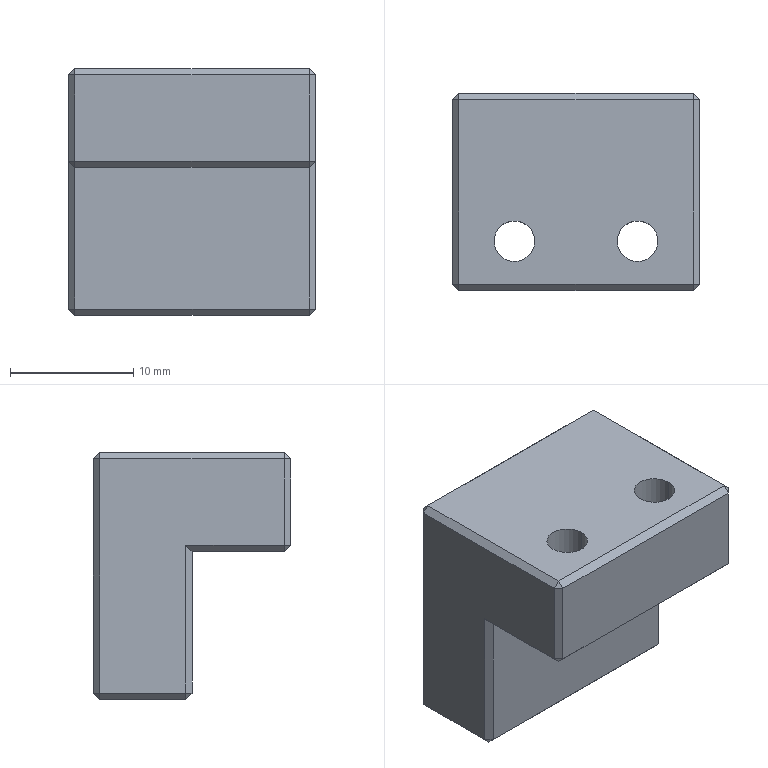Part | SolidWorks | features HoleWzd 2, Chamfer 1, Extrusion 1, ICE 1 | 1 solid | 47 faces | box 20 x 16 x 20 mm | volume 4067 mm3 | plane 35 | cylinder 8 | cone 4 | commonest cylinder face diameters 3.3 x8
STEP:
#1=CARTESIAN_POINT('',(-6.65,-4.,2.));
#2=VERTEX_POINT('',#1);
#3=CARTESIAN_POINT('',(-3.35,-4.,2.));
#4=VERTEX_POINT('',#3);
#5=CARTESIAN_POINT('',(-5.,-4.,2.));
#6=DIRECTION('',(0.,0.,1.));
#7=DIRECTION('',(1.,0.,0.));
#8=AXIS2_PLACEMENT_3D('',#5,#6,#7);
#9=CIRCLE('',#8,1.65);
#10=EDGE_CURVE('',#2,#4,#9,.T.);
#11=ORIENTED_EDGE('',*,*,#10,.F.);
#12=CARTESIAN_POINT('',(-6.65,-4.,10.));
#13=VERTEX_POINT('',#12);
#14=CARTESIAN_POINT('',(-6.65,-4.,10.));
#15=DIRECTION('',(0.,0.,1.));
#16=VECTOR('',#15,1000.);
#17=LINE('',#14,#16);
#18=EDGE_CURVE('',#2,#13,#17,.T.);
#19=ORIENTED_EDGE('',*,*,#18,.T.);
#20=CARTESIAN_POINT('',(-3.35,-4.,10.));
#21=VERTEX_POINT('',#20);
#22=CARTESIAN_POINT('',(-5.,-4.,10.));
#23=DIRECTION('',(0.,0.,1.));
#24=DIRECTION('',(1.,0.,0.));
#25=AXIS2_PLACEMENT_3D('',#22,#23,#24);
#26=CIRCLE('',#25,1.65);
#27=EDGE_CURVE('',#13,#21,#26,.T.);
#28=ORIENTED_EDGE('',*,*,#27,.T.);
#29=CARTESIAN_POINT('',(-3.35,-4.,10.));
#30=DIRECTION('',(0.,0.,1.));
#31=VECTOR('',#30,1000.);
#32=LINE('',#29,#31);
#33=EDGE_CURVE('',#4,#21,#32,.T.);
#34=ORIENTED_EDGE('',*,*,#33,.F.);
#35=EDGE_LOOP('',(#11,#19,#28,#34));
#36=FACE_OUTER_BOUND('',#35,.T.);
#37=CARTESIAN_POINT('',(-5.,-4.,10.));
#38=DIRECTION('',(0.,0.,1.));
#39=DIRECTION('',(1.,0.,0.));
#40=AXIS2_PLACEMENT_3D('',#37,#38,#39);
#41=CYLINDRICAL_SURFACE('',#40,1.65);
#42=ADVANCED_FACE('',(#36),#41,.F.);
#43=CARTESIAN_POINT('',(3.35,-4.,2.));
#44=VERTEX_POINT('',#43);
#45=CARTESIAN_POINT('',(6.65,-4.,2.));
#46=VERTEX_POINT('',#45);
#47=CARTESIAN_POINT('',(5.,-4.,2.));
#48=DIRECTION('',(0.,0.,1.));
#49=DIRECTION('',(1.,0.,0.));
#50=AXIS2_PLACEMENT_3D('',#47,#48,#49);
#51=CIRCLE('',#50,1.65);
#52=EDGE_CURVE('',#44,#46,#51,.T.);
#53=ORIENTED_EDGE('',*,*,#52,.F.);
#54=CARTESIAN_POINT('',(3.35,-4.,10.));
#55=VERTEX_POINT('',#54);
#56=CARTESIAN_POINT('',(3.35,-4.,10.));
#57=DIRECTION('',(0.,0.,1.));
#58=VECTOR('',#57,1000.);
#59=LINE('',#56,#58);
#60=EDGE_CURVE('',#44,#55,#59,.T.);
#61=ORIENTED_EDGE('',*,*,#60,.T.);
#62=CARTESIAN_POINT('',(6.65,-4.,10.));
#63=VERTEX_POINT('',#62);
#64=CARTESIAN_POINT('',(5.,-4.,10.));
#65=DIRECTION('',(0.,0.,1.));
#66=DIRECTION('',(1.,0.,0.));
#67=AXIS2_PLACEMENT_3D('',#64,#65,#66);
#68=CIRCLE('',#67,1.65);
#69=EDGE_CURVE('',#55,#63,#68,.T.);
#70=ORIENTED_EDGE('',*,*,#69,.T.);
#71=CARTESIAN_POINT('',(6.65,-4.,10.));
#72=DIRECTION('',(0.,0.,1.));
#73=VECTOR('',#72,1000.);
#74=LINE('',#71,#73);
#75=EDGE_CURVE('',#46,#63,#74,.T.);
#76=ORIENTED_EDGE('',*,*,#75,.F.);
#77=EDGE_LOOP('',(#53,#61,#70,#76));
#78=FACE_OUTER_BOUND('',#77,.T.);
#79=CARTESIAN_POINT('',(5.,-4.,10.));
#80=DIRECTION('',(0.,0.,1.));
#81=DIRECTION('',(1.,0.,0.));
#82=AXIS2_PLACEMENT_3D('',#79,#80,#81);
#83=CYLINDRICAL_SURFACE('',#82,1.65);
#84=ADVANCED_FACE('',(#78),#83,.F.);
#85=CARTESIAN_POINT('',(-4.1,4.,-3.35));
#86=VERTEX_POINT('',#85);
#87=CARTESIAN_POINT('',(-4.1,4.,-6.65));
#88=VERTEX_POINT('',#87);
#89=CARTESIAN_POINT('',(-4.1,4.,-5.));
#90=DIRECTION('',(1.,0.,0.));
#91=DIRECTION('',(0.,0.,-1.));
#92=AXIS2_PLACEMENT_3D('',#89,#90,#91);
#93=CIRCLE('',#92,1.65);
#94=EDGE_CURVE('',#86,#88,#93,.T.);
#95=ORIENTED_EDGE('',*,*,#94,.F.);
#96=CARTESIAN_POINT('',(10.,4.,-3.35));
#97=VERTEX_POINT('',#96);
#98=CARTESIAN_POINT('',(10.,4.,-3.35));
#99=DIRECTION('',(1.,0.,0.));
#100=VECTOR('',#99,1000.);
#101=LINE('',#98,#100);
#102=EDGE_CURVE('',#86,#97,#101,.T.);
#103=ORIENTED_EDGE('',*,*,#102,.T.);
#104=CARTESIAN_POINT('',(10.,4.,-6.65));
#105=VERTEX_POINT('',#104);
#106=CARTESIAN_POINT('',(10.,4.,-5.));
#107=DIRECTION('',(1.,0.,0.));
#108=DIRECTION('',(0.,0.,-1.));
#109=AXIS2_PLACEMENT_3D('',#106,#107,#108);
#110=CIRCLE('',#109,1.65);
#111=EDGE_CURVE('',#97,#105,#110,.T.);
#112=ORIENTED_EDGE('',*,*,#111,.T.);
#113=CARTESIAN_POINT('',(10.,4.,-6.65));
#114=DIRECTION('',(1.,0.,0.));
#115=VECTOR('',#114,1000.);
#116=LINE('',#113,#115);
#117=EDGE_CURVE('',#88,#105,#116,.T.);
#118=ORIENTED_EDGE('',*,*,#117,.F.);
#119=EDGE_LOOP('',(#95,#103,#112,#118));
#120=FACE_OUTER_BOUND('',#119,.T.);
#121=CARTESIAN_POINT('',(10.,4.,-5.));
#122=DIRECTION('',(1.,0.,0.));
#123=DIRECTION('',(0.,0.,-1.));
#124=AXIS2_PLACEMENT_3D('',#121,#122,#123);
#125=CYLINDRICAL_SURFACE('',#124,1.65);
#126=ADVANCED_FACE('',(#120),#125,.F.);
#127=CARTESIAN_POINT('',(-5.091,4.,-5.));
#128=VERTEX_POINT('',#127);
#129=CARTESIAN_POINT('',(-4.1,4.,-6.65));
#130=DIRECTION('',(0.515,0.,-0.8572));
#131=VECTOR('',#130,1000.);
#132=LINE('',#129,#131);
#133=EDGE_CURVE('',#128,#88,#132,.T.);
#134=ORIENTED_EDGE('',*,*,#133,.F.);
#135=CARTESIAN_POINT('',(-4.1,4.,-3.35));
#136=DIRECTION('',(0.515,0.,0.8572));
#137=VECTOR('',#136,1000.);
#138=LINE('',#135,#137);
#139=EDGE_CURVE('',#128,#86,#138,.T.);
#140=ORIENTED_EDGE('',*,*,#139,.T.);
#141=ORIENTED_EDGE('',*,*,#94,.T.);
#142=EDGE_LOOP('',(#134,#140,#141));
#143=FACE_OUTER_BOUND('',#142,.T.);
#144=CARTESIAN_POINT('',(-4.1,4.,-5.));
#145=DIRECTION('',(1.,0.,0.));
#146=DIRECTION('',(0.,0.,-1.));
#147=AXIS2_PLACEMENT_3D('',#144,#145,#146);
#148=CONICAL_SURFACE('',#147,1.65,1.03);
#149=ADVANCED_FACE('',(#143),#148,.F.);
#150=CARTESIAN_POINT('',(-4.1,4.,6.65));
#151=VERTEX_POINT('',#150);
#152=CARTESIAN_POINT('',(-4.1,4.,3.35));
#153=VERTEX_POINT('',#152);
#154=CARTESIAN_POINT('',(-4.1,4.,5.));
#155=DIRECTION('',(1.,0.,0.));
#156=DIRECTION('',(0.,0.,-1.));
#157=AXIS2_PLACEMENT_3D('',#154,#155,#156);
#158=CIRCLE('',#157,1.65);
#159=EDGE_CURVE('',#151,#153,#158,.T.);
#160=ORIENTED_EDGE('',*,*,#159,.F.);
#161=CARTESIAN_POINT('',(10.,4.,6.65));
#162=VERTEX_POINT('',#161);
#163=CARTESIAN_POINT('',(10.,4.,6.65));
#164=DIRECTION('',(1.,0.,0.));
#165=VECTOR('',#164,1000.);
#166=LINE('',#163,#165);
#167=EDGE_CURVE('',#151,#162,#166,.T.);
#168=ORIENTED_EDGE('',*,*,#167,.T.);
#169=CARTESIAN_POINT('',(10.,4.,3.35));
#170=VERTEX_POINT('',#169);
#171=CARTESIAN_POINT('',(10.,4.,5.));
#172=DIRECTION('',(1.,0.,0.));
#173=DIRECTION('',(0.,0.,-1.));
#174=AXIS2_PLACEMENT_3D('',#171,#172,#173);
#175=CIRCLE('',#174,1.65);
#176=EDGE_CURVE('',#162,#170,#175,.T.);
#177=ORIENTED_EDGE('',*,*,#176,.T.);
#178=CARTESIAN_POINT('',(10.,4.,3.35));
#179=DIRECTION('',(1.,0.,0.));
#180=VECTOR('',#179,1000.);
#181=LINE('',#178,#180);
#182=EDGE_CURVE('',#153,#170,#181,.T.);
#183=ORIENTED_EDGE('',*,*,#182,.F.);
#184=EDGE_LOOP('',(#160,#168,#177,#183));
#185=FACE_OUTER_BOUND('',#184,.T.);
#186=CARTESIAN_POINT('',(10.,4.,5.));
#187=DIRECTION('',(1.,0.,0.));
#188=DIRECTION('',(0.,0.,-1.));
#189=AXIS2_PLACEMENT_3D('',#186,#187,#188);
#190=CYLINDRICAL_SURFACE('',#189,1.65);
#191=ADVANCED_FACE('',(#185),#190,.F.);
#192=CARTESIAN_POINT('',(-5.091,4.,5.));
#193=VERTEX_POINT('',#192);
#194=CARTESIAN_POINT('',(-4.1,4.,3.35));
#195=DIRECTION('',(0.515,0.,-0.8572));
#196=VECTOR('',#195,1000.);
#197=LINE('',#194,#196);
#198=EDGE_CURVE('',#193,#153,#197,.T.);
#199=ORIENTED_EDGE('',*,*,#198,.F.);
#200=CARTESIAN_POINT('',(-4.1,4.,6.65));
#201=DIRECTION('',(0.515,0.,0.8572));
#202=VECTOR('',#201,1000.);
#203=LINE('',#200,#202);
#204=EDGE_CURVE('',#193,#151,#203,.T.);
#205=ORIENTED_EDGE('',*,*,#204,.T.);
#206=ORIENTED_EDGE('',*,*,#159,.T.);
#207=EDGE_LOOP('',(#199,#205,#206));
#208=FACE_OUTER_BOUND('',#207,.T.);
#209=CARTESIAN_POINT('',(-4.1,4.,5.));
#210=DIRECTION('',(1.,0.,0.));
#211=DIRECTION('',(0.,0.,-1.));
#212=AXIS2_PLACEMENT_3D('',#209,#210,#211);
#213=CONICAL_SURFACE('',#212,1.65,1.03);
#214=ADVANCED_FACE('',(#208),#213,.F.);
#215=CARTESIAN_POINT('',(10.,-7.5,2.5));
#216=VERTEX_POINT('',#215);
#217=CARTESIAN_POINT('',(10.,0.5,2.5));
#218=VERTEX_POINT('',#217);
#219=CARTESIAN_POINT('',(10.,8.,2.5));
#220=DIRECTION('',(0.,1.,0.));
#221=VECTOR('',#220,1000.);
#222=LINE('',#219,#221);
#223=EDGE_CURVE('',#216,#218,#222,.T.);
#224=ORIENTED_EDGE('',*,*,#223,.T.);
#225=CARTESIAN_POINT('',(10.,0.5,-9.5));
#226=VERTEX_POINT('',#225);
#227=CARTESIAN_POINT('',(10.,0.5,-10.));
#228=DIRECTION('',(0.,0.,-1.));
#229=VECTOR('',#228,1000.);
#230=LINE('',#227,#229);
#231=EDGE_CURVE('',#218,#226,#230,.T.);
#232=ORIENTED_EDGE('',*,*,#231,.T.);
#233=CARTESIAN_POINT('',(10.,7.5,-9.5));
#234=VERTEX_POINT('',#233);
#235=CARTESIAN_POINT('',(10.,8.,-9.5));
#236=DIRECTION('',(0.,1.,0.));
#237=VECTOR('',#236,1000.);
#238=LINE('',#235,#237);
#239=EDGE_CURVE('',#226,#234,#238,.T.);
#240=ORIENTED_EDGE('',*,*,#239,.T.);
#241=CARTESIAN_POINT('',(10.,7.5,9.5));
#242=VERTEX_POINT('',#241);
#243=CARTESIAN_POINT('',(10.,7.5,10.));
#244=DIRECTION('',(0.,0.,1.));
#245=VECTOR('',#244,1000.);
#246=LINE('',#243,#245);
#247=EDGE_CURVE('',#234,#242,#246,.T.);
#248=ORIENTED_EDGE('',*,*,#247,.T.);
#249=CARTESIAN_POINT('',(10.,-7.5,9.5));
#250=VERTEX_POINT('',#249);
#251=CARTESIAN_POINT('',(10.,8.,9.5));
#252=DIRECTION('',(0.,-1.,0.));
#253=VECTOR('',#252,1000.);
#254=LINE('',#251,#253);
#255=EDGE_CURVE('',#242,#250,#254,.T.);
#256=ORIENTED_EDGE('',*,*,#255,.T.);
#257=CARTESIAN_POINT('',(10.,-7.5,2.));
#258=DIRECTION('',(0.,0.,-1.));
#259=VECTOR('',#258,1000.);
#260=LINE('',#257,#259);
#261=EDGE_CURVE('',#250,#216,#260,.T.);
#262=ORIENTED_EDGE('',*,*,#261,.T.);
#263=EDGE_LOOP('',(#224,#232,#240,#248,#256,#262));
#264=FACE_OUTER_BOUND('',#263,.T.);
#265=CARTESIAN_POINT('',(10.,4.,-5.));
#266=DIRECTION('',(1.,0.,0.));
#267=DIRECTION('',(0.,0.,-1.));
#268=AXIS2_PLACEMENT_3D('',#265,#266,#267);
#269=CIRCLE('',#268,1.65);
#270=EDGE_CURVE('',#105,#97,#269,.T.);
#271=ORIENTED_EDGE('',*,*,#270,.F.);
#272=ORIENTED_EDGE('',*,*,#111,.F.);
#273=EDGE_LOOP('',(#271,#272));
#274=FACE_BOUND('',#273,.T.);
#275=CARTESIAN_POINT('',(10.,4.,5.));
#276=DIRECTION('',(1.,0.,0.));
#277=DIRECTION('',(0.,0.,-1.));
#278=AXIS2_PLACEMENT_3D('',#275,#276,#277);
#279=CIRCLE('',#278,1.65);
#280=EDGE_CURVE('',#170,#162,#279,.T.);
#281=ORIENTED_EDGE('',*,*,#280,.F.);
#282=ORIENTED_EDGE('',*,*,#176,.F.);
#283=EDGE_LOOP('',(#281,#282));
#284=FACE_BOUND('',#283,.T.);
#285=CARTESIAN_POINT('',(10.,8.,-10.));
#286=DIRECTION('',(-1.,0.,0.));
#287=DIRECTION('',(0.,0.,1.));
#288=AXIS2_PLACEMENT_3D('',#285,#286,#287);
#289=PLANE('',#288);
#290=ADVANCED_FACE('',(#264,#274,#284),#289,.F.);
#291=CARTESIAN_POINT('',(-9.5,7.5,-10.));
#292=VERTEX_POINT('',#291);
#293=CARTESIAN_POINT('',(9.5,7.5,-10.));
#294=VERTEX_POINT('',#293);
#295=CARTESIAN_POINT('',(10.,7.5,-10.));
#296=DIRECTION('',(1.,0.,0.));
#297=VECTOR('',#296,1000.);
#298=LINE('',#295,#297);
#299=EDGE_CURVE('',#292,#294,#298,.T.);
#300=ORIENTED_EDGE('',*,*,#299,.T.);
#301=CARTESIAN_POINT('',(9.5,0.5,-10.));
#302=VERTEX_POINT('',#301);
#303=CARTESIAN_POINT('',(9.5,8.,-10.));
#304=DIRECTION('',(0.,-1.,0.));
#305=VECTOR('',#304,1000.);
#306=LINE('',#303,#305);
#307=EDGE_CURVE('',#294,#302,#306,.T.);
#308=ORIENTED_EDGE('',*,*,#307,.T.);
#309=CARTESIAN_POINT('',(-9.5,0.5,-10.));
#310=VERTEX_POINT('',#309);
#311=CARTESIAN_POINT('',(-10.,0.5,-10.));
#312=DIRECTION('',(-1.,0.,0.));
#313=VECTOR('',#312,1000.);
#314=LINE('',#311,#313);
#315=EDGE_CURVE('',#302,#310,#314,.T.);
#316=ORIENTED_EDGE('',*,*,#315,.T.);
#317=CARTESIAN_POINT('',(-9.5,8.,-10.));
#318=DIRECTION('',(0.,1.,0.));
#319=VECTOR('',#318,1000.);
#320=LINE('',#317,#319);
#321=EDGE_CURVE('',#310,#292,#320,.T.);
#322=ORIENTED_EDGE('',*,*,#321,.T.);
#323=EDGE_LOOP('',(#300,#308,#316,#322));
#324=FACE_OUTER_BOUND('',#323,.T.);
#325=CARTESIAN_POINT('',(-10.,8.,-10.));
#326=DIRECTION('',(0.,0.,1.));
#327=DIRECTION('',(1.,0.,0.));
#328=AXIS2_PLACEMENT_3D('',#325,#326,#327);
#329=PLANE('',#328);
#330=ADVANCED_FACE('',(#324),#329,.F.);
#331=CARTESIAN_POINT('',(-10.,7.5,-9.5));
#332=VERTEX_POINT('',#331);
#333=CARTESIAN_POINT('',(-10.,0.5,-9.5));
#334=VERTEX_POINT('',#333);
#335=CARTESIAN_POINT('',(-10.,8.,-9.5));
#336=DIRECTION('',(0.,-1.,0.));
#337=VECTOR('',#336,1000.);
#338=LINE('',#335,#337);
#339=EDGE_CURVE('',#332,#334,#338,.T.);
#340=ORIENTED_EDGE('',*,*,#339,.T.);
#341=CARTESIAN_POINT('',(-10.,0.5,2.5));
#342=VERTEX_POINT('',#341);
#343=CARTESIAN_POINT('',(-10.,0.5,-10.));
#344=DIRECTION('',(0.,0.,1.));
#345=VECTOR('',#344,1000.);
#346=LINE('',#343,#345);
#347=EDGE_CURVE('',#334,#342,#346,.T.);
#348=ORIENTED_EDGE('',*,*,#347,.T.);
#349=CARTESIAN_POINT('',(-10.,-7.5,2.5));
#350=VERTEX_POINT('',#349);
#351=CARTESIAN_POINT('',(-10.,8.,2.5));
#352=DIRECTION('',(0.,-1.,0.));
#353=VECTOR('',#352,1000.);
#354=LINE('',#351,#353);
#355=EDGE_CURVE('',#342,#350,#354,.T.);
#356=ORIENTED_EDGE('',*,*,#355,.T.);
#357=CARTESIAN_POINT('',(-10.,-7.5,9.5));
#358=VERTEX_POINT('',#357);
#359=CARTESIAN_POINT('',(-10.,-7.5,10.));
#360=DIRECTION('',(0.,0.,1.));
#361=VECTOR('',#360,1000.);
#362=LINE('',#359,#361);
#363=EDGE_CURVE('',#350,#358,#362,.T.);
#364=ORIENTED_EDGE('',*,*,#363,.T.);
#365=CARTESIAN_POINT('',(-10.,7.5,9.5));
#366=VERTEX_POINT('',#365);
#367=CARTESIAN_POINT('',(-10.,8.,9.5));
#368=DIRECTION('',(0.,1.,0.));
#369=VECTOR('',#368,1000.);
#370=LINE('',#367,#369);
#371=EDGE_CURVE('',#358,#366,#370,.T.);
#372=ORIENTED_EDGE('',*,*,#371,.T.);
#373=CARTESIAN_POINT('',(-10.,7.5,-10.));
#374=DIRECTION('',(0.,0.,-1.));
#375=VECTOR('',#374,1000.);
#376=LINE('',#373,#375);
#377=EDGE_CURVE('',#366,#332,#376,.T.);
#378=ORIENTED_EDGE('',*,*,#377,.T.);
#379=EDGE_LOOP('',(#340,#348,#356,#364,#372,#378));
#380=FACE_OUTER_BOUND('',#379,.T.);
#381=CARTESIAN_POINT('',(-10.,8.,-10.));
#382=DIRECTION('',(1.,0.,0.));
#383=DIRECTION('',(0.,0.,-1.));
#384=AXIS2_PLACEMENT_3D('',#381,#382,#383);
#385=PLANE('',#384);
#386=ADVANCED_FACE('',(#380),#385,.F.);
#387=CARTESIAN_POINT('',(9.5,7.5,10.));
#388=VERTEX_POINT('',#387);
#389=CARTESIAN_POINT('',(-9.5,7.5,10.));
#390=VERTEX_POINT('',#389);
#391=CARTESIAN_POINT('',(-10.,7.5,10.));
#392=DIRECTION('',(-1.,0.,0.));
#393=VECTOR('',#392,1000.);
#394=LINE('',#391,#393);
#395=EDGE_CURVE('',#388,#390,#394,.T.);
#396=ORIENTED_EDGE('',*,*,#395,.T.);
#397=CARTESIAN_POINT('',(-9.5,-7.5,10.));
#398=VERTEX_POINT('',#397);
#399=CARTESIAN_POINT('',(-9.5,8.,10.));
#400=DIRECTION('',(0.,-1.,0.));
#401=VECTOR('',#400,1000.);
#402=LINE('',#399,#401);
#403=EDGE_CURVE('',#390,#398,#402,.T.);
#404=ORIENTED_EDGE('',*,*,#403,.T.);
#405=CARTESIAN_POINT('',(9.5,-7.5,10.));
#406=VERTEX_POINT('',#405);
#407=CARTESIAN_POINT('',(10.,-7.5,10.));
#408=DIRECTION('',(1.,0.,0.));
#409=VECTOR('',#408,1000.);
#410=LINE('',#407,#409);
#411=EDGE_CURVE('',#398,#406,#410,.T.);
#412=ORIENTED_EDGE('',*,*,#411,.T.);
#413=CARTESIAN_POINT('',(9.5,8.,10.));
#414=DIRECTION('',(0.,1.,0.));
#415=VECTOR('',#414,1000.);
#416=LINE('',#413,#415);
#417=EDGE_CURVE('',#406,#388,#416,.T.);
#418=ORIENTED_EDGE('',*,*,#417,.T.);
#419=EDGE_LOOP('',(#396,#404,#412,#418));
#420=FACE_OUTER_BOUND('',#419,.T.);
#421=CARTESIAN_POINT('',(-5.,-4.,10.));
#422=DIRECTION('',(0.,0.,1.));
#423=DIRECTION('',(1.,0.,0.));
#424=AXIS2_PLACEMENT_3D('',#421,#422,#423);
#425=CIRCLE('',#424,1.65);
#426=EDGE_CURVE('',#21,#13,#425,.T.);
#427=ORIENTED_EDGE('',*,*,#426,.F.);
#428=ORIENTED_EDGE('',*,*,#27,.F.);
#429=EDGE_LOOP('',(#427,#428));
#430=FACE_BOUND('',#429,.T.);
#431=CARTESIAN_POINT('',(5.,-4.,10.));
#432=DIRECTION('',(0.,0.,1.));
#433=DIRECTION('',(1.,0.,0.));
#434=AXIS2_PLACEMENT_3D('',#431,#432,#433);
#435=CIRCLE('',#434,1.65);
#436=EDGE_CURVE('',#63,#55,#435,.T.);
#437=ORIENTED_EDGE('',*,*,#436,.F.);
#438=ORIENTED_EDGE('',*,*,#69,.F.);
#439=EDGE_LOOP('',(#437,#438));
#440=FACE_BOUND('',#439,.T.);
#441=CARTESIAN_POINT('',(-10.,8.,10.));
#442=DIRECTION('',(0.,0.,-1.));
#443=DIRECTION('',(-1.,0.,0.));
#444=AXIS2_PLACEMENT_3D('',#441,#442,#443);
#445=PLANE('',#444);
#446=ADVANCED_FACE('',(#420,#430,#440),#445,.F.);
#447=CARTESIAN_POINT('',(9.5,8.,-9.5));
#448=VERTEX_POINT('',#447);
#449=CARTESIAN_POINT('',(-9.5,8.,-9.5));
#450=VERTEX_POINT('',#449);
#451=CARTESIAN_POINT('',(-10.,8.,-9.5));
#452=DIRECTION('',(-1.,0.,0.));
#453=VECTOR('',#452,1000.);
#454=LINE('',#451,#453);
#455=EDGE_CURVE('',#448,#450,#454,.T.);
#456=ORIENTED_EDGE('',*,*,#455,.T.);
#457=CARTESIAN_POINT('',(-9.5,8.,9.5));
#458=VERTEX_POINT('',#457);
#459=CARTESIAN_POINT('',(-9.5,8.,10.));
#460=DIRECTION('',(0.,0.,1.));
#461=VECTOR('',#460,1000.);
#462=LINE('',#459,#461);
#463=EDGE_CURVE('',#450,#458,#462,.T.);
#464=ORIENTED_EDGE('',*,*,#463,.T.);
#465=CARTESIAN_POINT('',(9.5,8.,9.5));
#466=VERTEX_POINT('',#465);
#467=CARTESIAN_POINT('',(10.,8.,9.5));
#468=DIRECTION('',(1.,0.,0.));
#469=VECTOR('',#468,1000.);
#470=LINE('',#467,#469);
#471=EDGE_CURVE('',#458,#466,#470,.T.);
#472=ORIENTED_EDGE('',*,*,#471,.T.);
#473=CARTESIAN_POINT('',(9.5,8.,-10.));
#474=DIRECTION('',(0.,0.,-1.));
#475=VECTOR('',#474,1000.);
#476=LINE('',#473,#475);
#477=EDGE_CURVE('',#466,#448,#476,.T.);
#478=ORIENTED_EDGE('',*,*,#477,.T.);
#479=EDGE_LOOP('',(#456,#464,#472,#478));
#480=FACE_OUTER_BOUND('',#479,.T.);
#481=CARTESIAN_POINT('',(0.,8.,0.));
#482=DIRECTION('',(0.,1.,0.));
#483=DIRECTION('',(0.,0.,1.));
#484=AXIS2_PLACEMENT_3D('',#481,#482,#483);
#485=PLANE('',#484);
#486=ADVANCED_FACE('',(#480),#485,.T.);
#487=CARTESIAN_POINT('',(9.5,0.,2.));
#488=VERTEX_POINT('',#487);
#489=CARTESIAN_POINT('',(-9.5,0.,2.));
#490=VERTEX_POINT('',#489);
#491=CARTESIAN_POINT('',(-10.,0.,2.));
#492=DIRECTION('',(-1.,0.,0.));
#493=VECTOR('',#492,1000.);
#494=LINE('',#491,#493);
#495=EDGE_CURVE('',#488,#490,#494,.T.);
#496=ORIENTED_EDGE('',*,*,#495,.T.);
#497=CARTESIAN_POINT('',(-9.5,0.,-9.5));
#498=VERTEX_POINT('',#497);
#499=CARTESIAN_POINT('',(-9.5,0.,0.));
#500=DIRECTION('',(0.,0.,-1.));
#501=VECTOR('',#500,1000.);
#502=LINE('',#499,#501);
#503=EDGE_CURVE('',#490,#498,#502,.T.);
#504=ORIENTED_EDGE('',*,*,#503,.T.);
#505=CARTESIAN_POINT('',(9.5,0.,-9.5));
#506=VERTEX_POINT('',#505);
#507=CARTESIAN_POINT('',(0.,0.,-9.5));
#508=DIRECTION('',(1.,0.,0.));
#509=VECTOR('',#508,1000.);
#510=LINE('',#507,#509);
#511=EDGE_CURVE('',#498,#506,#510,.T.);
#512=ORIENTED_EDGE('',*,*,#511,.T.);
#513=CARTESIAN_POINT('',(9.5,0.,0.));
#514=DIRECTION('',(0.,0.,1.));
#515=VECTOR('',#514,1000.);
#516=LINE('',#513,#515);
#517=EDGE_CURVE('',#506,#488,#516,.T.);
#518=ORIENTED_EDGE('',*,*,#517,.T.);
#519=EDGE_LOOP('',(#496,#504,#512,#518));
#520=FACE_OUTER_BOUND('',#519,.T.);
#521=CARTESIAN_POINT('',(0.,0.,0.));
#522=DIRECTION('',(0.,1.,0.));
#523=DIRECTION('',(0.,0.,1.));
#524=AXIS2_PLACEMENT_3D('',#521,#522,#523);
#525=PLANE('',#524);
#526=ADVANCED_FACE('',(#520),#525,.F.);
#527=ORIENTED_EDGE('',*,*,#204,.F.);
#528=ORIENTED_EDGE('',*,*,#198,.T.);
#529=CARTESIAN_POINT('',(-4.1,4.,5.));
#530=DIRECTION('',(1.,0.,0.));
#531=DIRECTION('',(0.,0.,-1.));
#532=AXIS2_PLACEMENT_3D('',#529,#530,#531);
#533=CIRCLE('',#532,1.65);
#534=EDGE_CURVE('',#153,#151,#533,.T.);
#535=ORIENTED_EDGE('',*,*,#534,.T.);
#536=EDGE_LOOP('',(#527,#528,#535));
#537=FACE_OUTER_BOUND('',#536,.T.);
#538=CARTESIAN_POINT('',(-4.1,4.,5.));
#539=DIRECTION('',(1.,0.,0.));
#540=DIRECTION('',(0.,0.,-1.));
#541=AXIS2_PLACEMENT_3D('',#538,#539,#540);
#542=CONICAL_SURFACE('',#541,1.65,1.03);
#543=ADVANCED_FACE('',(#537),#542,.F.);
#544=ORIENTED_EDGE('',*,*,#167,.F.);
#545=ORIENTED_EDGE('',*,*,#534,.F.);
#546=ORIENTED_EDGE('',*,*,#182,.T.);
#547=ORIENTED_EDGE('',*,*,#280,.T.);
#548=EDGE_LOOP('',(#544,#545,#546,#547));
#549=FACE_OUTER_BOUND('',#548,.T.);
#550=CARTESIAN_POINT('',(10.,4.,5.));
#551=DIRECTION('',(1.,0.,0.));
#552=DIRECTION('',(0.,0.,-1.));
#553=AXIS2_PLACEMENT_3D('',#550,#551,#552);
#554=CYLINDRICAL_SURFACE('',#553,1.65);
#555=ADVANCED_FACE('',(#549),#554,.F.);
#556=ORIENTED_EDGE('',*,*,#139,.F.);
#557=ORIENTED_EDGE('',*,*,#133,.T.);
#558=CARTESIAN_POINT('',(-4.1,4.,-5.));
#559=DIRECTION('',(1.,0.,0.));
#560=DIRECTION('',(0.,0.,-1.));
#561=AXIS2_PLACEMENT_3D('',#558,#559,#560);
#562=CIRCLE('',#561,1.65);
#563=EDGE_CURVE('',#88,#86,#562,.T.);
#564=ORIENTED_EDGE('',*,*,#563,.T.);
#565=EDGE_LOOP('',(#556,#557,#564));
#566=FACE_OUTER_BOUND('',#565,.T.);
#567=CARTESIAN_POINT('',(-4.1,4.,-5.));
#568=DIRECTION('',(1.,0.,0.));
#569=DIRECTION('',(0.,0.,-1.));
#570=AXIS2_PLACEMENT_3D('',#567,#568,#569);
#571=CONICAL_SURFACE('',#570,1.65,1.03);
#572=ADVANCED_FACE('',(#566),#571,.F.);
#573=ORIENTED_EDGE('',*,*,#102,.F.);
#574=ORIENTED_EDGE('',*,*,#563,.F.);
#575=ORIENTED_EDGE('',*,*,#117,.T.);
#576=ORIENTED_EDGE('',*,*,#270,.T.);
#577=EDGE_LOOP('',(#573,#574,#575,#576));
#578=FACE_OUTER_BOUND('',#577,.T.);
#579=CARTESIAN_POINT('',(10.,4.,-5.));
#580=DIRECTION('',(1.,0.,0.));
#581=DIRECTION('',(0.,0.,-1.));
#582=AXIS2_PLACEMENT_3D('',#579,#580,#581);
#583=CYLINDRICAL_SURFACE('',#582,1.65);
#584=ADVANCED_FACE('',(#578),#583,.F.);
#585=CARTESIAN_POINT('',(-9.5,-8.,2.5));
#586=VERTEX_POINT('',#585);
#587=CARTESIAN_POINT('',(9.5,-8.,2.5));
#588=VERTEX_POINT('',#587);
#589=CARTESIAN_POINT('',(10.,-8.,2.5));
#590=DIRECTION('',(1.,0.,0.));
#591=VECTOR('',#590,1000.);
#592=LINE('',#589,#591);
#593=EDGE_CURVE('',#586,#588,#592,.T.);
#594=ORIENTED_EDGE('',*,*,#593,.T.);
#595=CARTESIAN_POINT('',(9.5,-8.,9.5));
#596=VERTEX_POINT('',#595);
#597=CARTESIAN_POINT('',(9.5,-8.,10.));
#598=DIRECTION('',(0.,0.,1.));
#599=VECTOR('',#598,1000.);
#600=LINE('',#597,#599);
#601=EDGE_CURVE('',#588,#596,#600,.T.);
#602=ORIENTED_EDGE('',*,*,#601,.T.);
#603=CARTESIAN_POINT('',(-9.5,-8.,9.5));
#604=VERTEX_POINT('',#603);
#605=CARTESIAN_POINT('',(-10.,-8.,9.5));
#606=DIRECTION('',(-1.,0.,0.));
#607=VECTOR('',#606,1000.);
#608=LINE('',#605,#607);
#609=EDGE_CURVE('',#596,#604,#608,.T.);
#610=ORIENTED_EDGE('',*,*,#609,.T.);
#611=CARTESIAN_POINT('',(-9.5,-8.,2.));
#612=DIRECTION('',(0.,0.,-1.));
#613=VECTOR('',#612,1000.);
#614=LINE('',#611,#613);
#615=EDGE_CURVE('',#604,#586,#614,.T.);
#616=ORIENTED_EDGE('',*,*,#615,.T.);
#617=EDGE_LOOP('',(#594,#602,#610,#616));
#618=FACE_OUTER_BOUND('',#617,.T.);
#619=CARTESIAN_POINT('',(-10.,-8.,2.));
#620=DIRECTION('',(0.,-1.,0.));
#621=DIRECTION('',(0.,0.,-1.));
#622=AXIS2_PLACEMENT_3D('',#619,#620,#621);
#623=PLANE('',#622);
#624=ADVANCED_FACE('',(#618),#623,.T.);
#625=CARTESIAN_POINT('',(-5.,-4.,2.));
#626=DIRECTION('',(0.,0.,1.));
#627=DIRECTION('',(1.,0.,0.));
#628=AXIS2_PLACEMENT_3D('',#625,#626,#627);
#629=CIRCLE('',#628,1.65);
#630=EDGE_CURVE('',#4,#2,#629,.T.);
#631=ORIENTED_EDGE('',*,*,#630,.T.);
#632=ORIENTED_EDGE('',*,*,#10,.T.);
#633=EDGE_LOOP('',(#631,#632));
#634=FACE_BOUND('',#633,.T.);
#635=CARTESIAN_POINT('',(5.,-4.,2.));
#636=DIRECTION('',(0.,0.,1.));
#637=DIRECTION('',(1.,0.,0.));
#638=AXIS2_PLACEMENT_3D('',#635,#636,#637);
#639=CIRCLE('',#638,1.65);
#640=EDGE_CURVE('',#46,#44,#639,.T.);
#641=ORIENTED_EDGE('',*,*,#640,.T.);
#642=ORIENTED_EDGE('',*,*,#52,.T.);
#643=EDGE_LOOP('',(#641,#642));
#644=FACE_BOUND('',#643,.T.);
#645=CARTESIAN_POINT('',(9.5,-7.5,2.));
#646=VERTEX_POINT('',#645);
#647=CARTESIAN_POINT('',(-9.5,-7.5,2.));
#648=VERTEX_POINT('',#647);
#649=CARTESIAN_POINT('',(-10.,-7.5,2.));
#650=DIRECTION('',(-1.,0.,0.));
#651=VECTOR('',#650,1000.);
#652=LINE('',#649,#651);
#653=EDGE_CURVE('',#646,#648,#652,.T.);
#654=ORIENTED_EDGE('',*,*,#653,.T.);
#655=CARTESIAN_POINT('',(-9.5,0.,2.));
#656=DIRECTION('',(0.,1.,0.));
#657=VECTOR('',#656,1000.);
#658=LINE('',#655,#657);
#659=EDGE_CURVE('',#648,#490,#658,.T.);
#660=ORIENTED_EDGE('',*,*,#659,.T.);
#661=ORIENTED_EDGE('',*,*,#495,.F.);
#662=CARTESIAN_POINT('',(9.5,0.,2.));
#663=DIRECTION('',(0.,-1.,0.));
#664=VECTOR('',#663,1000.);
#665=LINE('',#662,#664);
#666=EDGE_CURVE('',#488,#646,#665,.T.);
#667=ORIENTED_EDGE('',*,*,#666,.T.);
#668=EDGE_LOOP('',(#654,#660,#661,#667));
#669=FACE_OUTER_BOUND('',#668,.T.);
#670=CARTESIAN_POINT('',(0.,0.,2.));
#671=DIRECTION('',(0.,0.,1.));
#672=DIRECTION('',(1.,0.,0.));
#673=AXIS2_PLACEMENT_3D('',#670,#671,#672);
#674=PLANE('',#673);
#675=ADVANCED_FACE('',(#634,#644,#669),#674,.F.);
#676=ORIENTED_EDGE('',*,*,#60,.F.);
#677=ORIENTED_EDGE('',*,*,#640,.F.);
#678=ORIENTED_EDGE('',*,*,#75,.T.);
#679=ORIENTED_EDGE('',*,*,#436,.T.);
#680=EDGE_LOOP('',(#676,#677,#678,#679));
#681=FACE_OUTER_BOUND('',#680,.T.);
#682=CARTESIAN_POINT('',(5.,-4.,10.));
#683=DIRECTION('',(0.,0.,1.));
#684=DIRECTION('',(1.,0.,0.));
#685=AXIS2_PLACEMENT_3D('',#682,#683,#684);
#686=CYLINDRICAL_SURFACE('',#685,1.65);
#687=ADVANCED_FACE('',(#681),#686,.F.);
#688=ORIENTED_EDGE('',*,*,#18,.F.);
#689=ORIENTED_EDGE('',*,*,#630,.F.);
#690=ORIENTED_EDGE('',*,*,#33,.T.);
#691=ORIENTED_EDGE('',*,*,#426,.T.);
#692=EDGE_LOOP('',(#688,#689,#690,#691));
#693=FACE_OUTER_BOUND('',#692,.T.);
#694=CARTESIAN_POINT('',(-5.,-4.,10.));
#695=DIRECTION('',(0.,0.,1.));
#696=DIRECTION('',(1.,0.,0.));
#697=AXIS2_PLACEMENT_3D('',#694,#695,#696);
#698=CYLINDRICAL_SURFACE('',#697,1.65);
#699=ADVANCED_FACE('',(#693),#698,.F.);
#700=CARTESIAN_POINT('',(10.,-7.5,2.5));
#701=DIRECTION('',(0.7071,0.,0.7071));
#702=VECTOR('',#701,1000.);
#703=LINE('',#700,#702);
#704=EDGE_CURVE('',#646,#216,#703,.T.);
#705=ORIENTED_EDGE('',*,*,#704,.F.);
#706=ORIENTED_EDGE('',*,*,#666,.F.);
#707=CARTESIAN_POINT('',(5.833,-3.667,-1.667));
#708=DIRECTION('',(-0.5774,-0.5774,-0.5774));
#709=VECTOR('',#708,1000.);
#710=LINE('',#707,#709);
#711=EDGE_CURVE('',#218,#488,#710,.T.);
#712=ORIENTED_EDGE('',*,*,#711,.F.);
#713=ORIENTED_EDGE('',*,*,#223,.F.);
#714=EDGE_LOOP('',(#705,#706,#712,#713));
#715=FACE_OUTER_BOUND('',#714,.T.);
#716=CARTESIAN_POINT('',(10.,8.,2.5));
#717=DIRECTION('',(-0.7071,0.,0.7071));
#718=DIRECTION('',(0.,1.,0.));
#719=AXIS2_PLACEMENT_3D('',#716,#717,#718);
#720=PLANE('',#719);
#721=ADVANCED_FACE('',(#715),#720,.F.);
#722=CARTESIAN_POINT('',(9.5,-7.75,2.25));
#723=DIRECTION('',(0.,-0.7071,0.7071));
#724=VECTOR('',#723,1000.);
#725=LINE('',#722,#724);
#726=EDGE_CURVE('',#646,#588,#725,.T.);
#727=ORIENTED_EDGE('',*,*,#726,.F.);
#728=ORIENTED_EDGE('',*,*,#704,.T.);
#729=CARTESIAN_POINT('',(10.,-7.5,2.5));
#730=DIRECTION('',(0.7071,0.7071,0.));
#731=VECTOR('',#730,1000.);
#732=LINE('',#729,#731);
#733=EDGE_CURVE('',#588,#216,#732,.T.);
#734=ORIENTED_EDGE('',*,*,#733,.F.);
#735=EDGE_LOOP('',(#727,#728,#734));
#736=FACE_OUTER_BOUND('',#735,.T.);
#737=CARTESIAN_POINT('',(10.,-7.5,2.5));
#738=DIRECTION('',(0.5774,-0.5774,-0.5774));
#739=DIRECTION('',(-0.7071,0.,-0.7071));
#740=AXIS2_PLACEMENT_3D('',#737,#738,#739);
#741=PLANE('',#740);
#742=ADVANCED_FACE('',(#736),#741,.T.);
#743=ORIENTED_EDGE('',*,*,#711,.T.);
#744=ORIENTED_EDGE('',*,*,#517,.F.);
#745=CARTESIAN_POINT('',(9.75,0.25,-9.5));
#746=DIRECTION('',(-0.7071,-0.7071,0.));
#747=VECTOR('',#746,1000.);
#748=LINE('',#745,#747);
#749=EDGE_CURVE('',#226,#506,#748,.T.);
#750=ORIENTED_EDGE('',*,*,#749,.F.);
#751=ORIENTED_EDGE('',*,*,#231,.F.);
#752=EDGE_LOOP('',(#743,#744,#750,#751));
#753=FACE_OUTER_BOUND('',#752,.T.);
#754=CARTESIAN_POINT('',(10.,0.5,-10.));
#755=DIRECTION('',(-0.7071,0.7071,0.));
#756=DIRECTION('',(0.,0.,-1.));
#757=AXIS2_PLACEMENT_3D('',#754,#755,#756);
#758=PLANE('',#757);
#759=ADVANCED_FACE('',(#753),#758,.F.);
#760=ORIENTED_EDGE('',*,*,#733,.T.);
#761=ORIENTED_EDGE('',*,*,#261,.F.);
#762=CARTESIAN_POINT('',(9.5,-8.,9.5));
#763=DIRECTION('',(0.7071,0.7071,0.));
#764=VECTOR('',#763,1000.);
#765=LINE('',#762,#764);
#766=EDGE_CURVE('',#596,#250,#765,.T.);
#767=ORIENTED_EDGE('',*,*,#766,.F.);
#768=ORIENTED_EDGE('',*,*,#601,.F.);
#769=EDGE_LOOP('',(#760,#761,#767,#768));
#770=FACE_OUTER_BOUND('',#769,.T.);
#771=CARTESIAN_POINT('',(9.5,-8.,2.));
#772=DIRECTION('',(0.7071,-0.7071,0.));
#773=DIRECTION('',(0.,0.,-1.));
#774=AXIS2_PLACEMENT_3D('',#771,#772,#773);
#775=PLANE('',#774);
#776=ADVANCED_FACE('',(#770),#775,.T.);
#777=ORIENTED_EDGE('',*,*,#726,.T.);
#778=ORIENTED_EDGE('',*,*,#593,.F.);
#779=CARTESIAN_POINT('',(-9.5,-7.75,2.25));
#780=DIRECTION('',(0.,-0.7071,0.7071));
#781=VECTOR('',#780,1000.);
#782=LINE('',#779,#781);
#783=EDGE_CURVE('',#648,#586,#782,.T.);
#784=ORIENTED_EDGE('',*,*,#783,.F.);
#785=ORIENTED_EDGE('',*,*,#653,.F.);
#786=EDGE_LOOP('',(#777,#778,#784,#785));
#787=FACE_OUTER_BOUND('',#786,.T.);
#788=CARTESIAN_POINT('',(-10.,-8.,2.5));
#789=DIRECTION('',(0.,-0.7071,-0.7071));
#790=DIRECTION('',(-1.,0.,0.));
#791=AXIS2_PLACEMENT_3D('',#788,#789,#790);
#792=PLANE('',#791);
#793=ADVANCED_FACE('',(#787),#792,.T.);
#794=CARTESIAN_POINT('',(-12.5,3.,5.));
#795=DIRECTION('',(-0.5774,0.5774,0.5774));
#796=VECTOR('',#795,1000.);
#797=LINE('',#794,#796);
#798=EDGE_CURVE('',#490,#342,#797,.T.);
#799=ORIENTED_EDGE('',*,*,#798,.F.);
#800=ORIENTED_EDGE('',*,*,#659,.F.);
#801=CARTESIAN_POINT('',(-10.,-7.5,2.5));
#802=DIRECTION('',(0.7071,0.,-0.7071));
#803=VECTOR('',#802,1000.);
#804=LINE('',#801,#803);
#805=EDGE_CURVE('',#350,#648,#804,.T.);
#806=ORIENTED_EDGE('',*,*,#805,.F.);
#807=ORIENTED_EDGE('',*,*,#355,.F.);
#808=EDGE_LOOP('',(#799,#800,#806,#807));
#809=FACE_OUTER_BOUND('',#808,.T.);
#810=CARTESIAN_POINT('',(-10.,8.,2.5));
#811=DIRECTION('',(0.7071,0.,0.7071));
#812=DIRECTION('',(0.,-1.,0.));
#813=AXIS2_PLACEMENT_3D('',#810,#811,#812);
#814=PLANE('',#813);
#815=ADVANCED_FACE('',(#809),#814,.F.);
#816=CARTESIAN_POINT('',(9.5,0.5,-10.));
#817=DIRECTION('',(-0.7071,0.,-0.7071));
#818=VECTOR('',#817,1000.);
#819=LINE('',#816,#818);
#820=EDGE_CURVE('',#226,#302,#819,.T.);
#821=ORIENTED_EDGE('',*,*,#820,.F.);
#822=ORIENTED_EDGE('',*,*,#749,.T.);
#823=CARTESIAN_POINT('',(9.5,0.5,-10.));
#824=DIRECTION('',(0.,-0.7071,0.7071));
#825=VECTOR('',#824,1000.);
#826=LINE('',#823,#825);
#827=EDGE_CURVE('',#302,#506,#826,.T.);
#828=ORIENTED_EDGE('',*,*,#827,.F.);
#829=EDGE_LOOP('',(#821,#822,#828));
#830=FACE_OUTER_BOUND('',#829,.T.);
#831=CARTESIAN_POINT('',(9.5,0.5,-10.));
#832=DIRECTION('',(0.5774,-0.5774,-0.5774));
#833=DIRECTION('',(0.,0.7071,-0.7071));
#834=AXIS2_PLACEMENT_3D('',#831,#832,#833);
#835=PLANE('',#834);
#836=ADVANCED_FACE('',(#830),#835,.T.);
#837=CARTESIAN_POINT('',(9.5,-8.,9.5));
#838=DIRECTION('',(0.,0.7071,0.7071));
#839=VECTOR('',#838,1000.);
#840=LINE('',#837,#839);
#841=EDGE_CURVE('',#596,#406,#840,.T.);
#842=ORIENTED_EDGE('',*,*,#841,.F.);
#843=ORIENTED_EDGE('',*,*,#766,.T.);
#844=CARTESIAN_POINT('',(9.75,-7.5,9.75));
#845=DIRECTION('',(0.7071,0.,-0.7071));
#846=VECTOR('',#845,1000.);
#847=LINE('',#844,#846);
#848=EDGE_CURVE('',#406,#250,#847,.T.);
#849=ORIENTED_EDGE('',*,*,#848,.F.);
#850=EDGE_LOOP('',(#842,#843,#849));
#851=FACE_OUTER_BOUND('',#850,.T.);
#852=CARTESIAN_POINT('',(9.5,-8.,9.5));
#853=DIRECTION('',(0.5774,-0.5774,0.5774));
#854=DIRECTION('',(0.7071,0.,-0.7071));
#855=AXIS2_PLACEMENT_3D('',#852,#853,#854);
#856=PLANE('',#855);
#857=ADVANCED_FACE('',(#851),#856,.T.);
#858=ORIENTED_EDGE('',*,*,#805,.T.);
#859=ORIENTED_EDGE('',*,*,#783,.T.);
#860=CARTESIAN_POINT('',(-10.,-7.5,2.5));
#861=DIRECTION('',(0.7071,-0.7071,0.));
#862=VECTOR('',#861,1000.);
#863=LINE('',#860,#862);
#864=EDGE_CURVE('',#350,#586,#863,.T.);
#865=ORIENTED_EDGE('',*,*,#864,.F.);
#866=EDGE_LOOP('',(#858,#859,#865));
#867=FACE_OUTER_BOUND('',#866,.T.);
#868=CARTESIAN_POINT('',(-10.,-7.5,2.5));
#869=DIRECTION('',(-0.5774,-0.5774,-0.5774));
#870=DIRECTION('',(0.,0.7071,-0.7071));
#871=AXIS2_PLACEMENT_3D('',#868,#869,#870);
#872=PLANE('',#871);
#873=ADVANCED_FACE('',(#867),#872,.T.);
#874=ORIENTED_EDGE('',*,*,#798,.T.);
#875=ORIENTED_EDGE('',*,*,#347,.F.);
#876=CARTESIAN_POINT('',(-9.5,0.,-9.5));
#877=DIRECTION('',(-0.7071,0.7071,0.));
#878=VECTOR('',#877,1000.);
#879=LINE('',#876,#878);
#880=EDGE_CURVE('',#498,#334,#879,.T.);
#881=ORIENTED_EDGE('',*,*,#880,.F.);
#882=ORIENTED_EDGE('',*,*,#503,.F.);
#883=EDGE_LOOP('',(#874,#875,#881,#882));
#884=FACE_OUTER_BOUND('',#883,.T.);
#885=CARTESIAN_POINT('',(-10.,0.5,-10.));
#886=DIRECTION('',(0.7071,0.7071,0.));
#887=DIRECTION('',(0.,0.,1.));
#888=AXIS2_PLACEMENT_3D('',#885,#886,#887);
#889=PLANE('',#888);
#890=ADVANCED_FACE('',(#884),#889,.F.);
#891=ORIENTED_EDGE('',*,*,#827,.T.);
#892=ORIENTED_EDGE('',*,*,#511,.F.);
#893=CARTESIAN_POINT('',(-9.5,0.,-9.5));
#894=DIRECTION('',(0.,-0.7071,0.7071));
#895=VECTOR('',#894,1000.);
#896=LINE('',#893,#895);
#897=EDGE_CURVE('',#310,#498,#896,.T.);
#898=ORIENTED_EDGE('',*,*,#897,.F.);
#899=ORIENTED_EDGE('',*,*,#315,.F.);
#900=EDGE_LOOP('',(#891,#892,#898,#899));
#901=FACE_OUTER_BOUND('',#900,.T.);
#902=CARTESIAN_POINT('',(-10.,0.5,-10.));
#903=DIRECTION('',(0.,0.7071,0.7071));
#904=DIRECTION('',(-1.,0.,0.));
#905=AXIS2_PLACEMENT_3D('',#902,#903,#904);
#906=PLANE('',#905);
#907=ADVANCED_FACE('',(#901),#906,.F.);
#908=ORIENTED_EDGE('',*,*,#820,.T.);
#909=ORIENTED_EDGE('',*,*,#307,.F.);
#910=CARTESIAN_POINT('',(10.,7.5,-9.5));
#911=DIRECTION('',(-0.7071,0.,-0.7071));
#912=VECTOR('',#911,1000.);
#913=LINE('',#910,#912);
#914=EDGE_CURVE('',#234,#294,#913,.T.);
#915=ORIENTED_EDGE('',*,*,#914,.F.);
#916=ORIENTED_EDGE('',*,*,#239,.F.);
#917=EDGE_LOOP('',(#908,#909,#915,#916));
#918=FACE_OUTER_BOUND('',#917,.T.);
#919=CARTESIAN_POINT('',(9.5,8.,-10.));
#920=DIRECTION('',(-0.7071,0.,0.7071));
#921=DIRECTION('',(0.,-1.,0.));
#922=AXIS2_PLACEMENT_3D('',#919,#920,#921);
#923=PLANE('',#922);
#924=ADVANCED_FACE('',(#918),#923,.F.);
#925=CARTESIAN_POINT('',(10.,7.5,9.5));
#926=DIRECTION('',(-0.7071,0.7071,0.));
#927=VECTOR('',#926,1000.);
#928=LINE('',#925,#927);
#929=EDGE_CURVE('',#242,#466,#928,.T.);
#930=ORIENTED_EDGE('',*,*,#929,.F.);
#931=ORIENTED_EDGE('',*,*,#247,.F.);
#932=CARTESIAN_POINT('',(10.,7.5,-9.5));
#933=DIRECTION('',(0.7071,-0.7071,0.));
#934=VECTOR('',#933,1000.);
#935=LINE('',#932,#934);
#936=EDGE_CURVE('',#448,#234,#935,.T.);
#937=ORIENTED_EDGE('',*,*,#936,.F.);
#938=ORIENTED_EDGE('',*,*,#477,.F.);
#939=EDGE_LOOP('',(#930,#931,#937,#938));
#940=FACE_OUTER_BOUND('',#939,.T.);
#941=CARTESIAN_POINT('',(9.5,8.,0.));
#942=DIRECTION('',(0.7071,0.7071,0.));
#943=DIRECTION('',(0.,0.,1.));
#944=AXIS2_PLACEMENT_3D('',#941,#942,#943);
#945=PLANE('',#944);
#946=ADVANCED_FACE('',(#940),#945,.T.);
#947=ORIENTED_EDGE('',*,*,#848,.T.);
#948=ORIENTED_EDGE('',*,*,#255,.F.);
#949=CARTESIAN_POINT('',(10.,7.5,9.5));
#950=DIRECTION('',(0.7071,0.,-0.7071));
#951=VECTOR('',#950,1000.);
#952=LINE('',#949,#951);
#953=EDGE_CURVE('',#388,#242,#952,.T.);
#954=ORIENTED_EDGE('',*,*,#953,.F.);
#955=ORIENTED_EDGE('',*,*,#417,.F.);
#956=EDGE_LOOP('',(#947,#948,#954,#955));
#957=FACE_OUTER_BOUND('',#956,.T.);
#958=CARTESIAN_POINT('',(10.,8.,9.5));
#959=DIRECTION('',(-0.7071,0.,-0.7071));
#960=DIRECTION('',(0.,-1.,0.));
#961=AXIS2_PLACEMENT_3D('',#958,#959,#960);
#962=PLANE('',#961);
#963=ADVANCED_FACE('',(#957),#962,.F.);
#964=ORIENTED_EDGE('',*,*,#841,.T.);
#965=ORIENTED_EDGE('',*,*,#411,.F.);
#966=CARTESIAN_POINT('',(-9.5,-7.5,10.));
#967=DIRECTION('',(0.,0.7071,0.7071));
#968=VECTOR('',#967,1000.);
#969=LINE('',#966,#968);
#970=EDGE_CURVE('',#604,#398,#969,.T.);
#971=ORIENTED_EDGE('',*,*,#970,.F.);
#972=ORIENTED_EDGE('',*,*,#609,.F.);
#973=EDGE_LOOP('',(#964,#965,#971,#972));
#974=FACE_OUTER_BOUND('',#973,.T.);
#975=CARTESIAN_POINT('',(-10.,-7.5,10.));
#976=DIRECTION('',(0.,-0.7071,0.7071));
#977=DIRECTION('',(-1.,0.,0.));
#978=AXIS2_PLACEMENT_3D('',#975,#976,#977);
#979=PLANE('',#978);
#980=ADVANCED_FACE('',(#974),#979,.T.);
#981=ORIENTED_EDGE('',*,*,#864,.T.);
#982=ORIENTED_EDGE('',*,*,#615,.F.);
#983=CARTESIAN_POINT('',(-9.75,-7.75,9.5));
#984=DIRECTION('',(0.7071,-0.7071,0.));
#985=VECTOR('',#984,1000.);
#986=LINE('',#983,#985);
#987=EDGE_CURVE('',#358,#604,#986,.T.);
#988=ORIENTED_EDGE('',*,*,#987,.F.);
#989=ORIENTED_EDGE('',*,*,#363,.F.);
#990=EDGE_LOOP('',(#981,#982,#988,#989));
#991=FACE_OUTER_BOUND('',#990,.T.);
#992=CARTESIAN_POINT('',(-10.,-7.5,-10.));
#993=DIRECTION('',(-0.7071,-0.7071,0.));
#994=DIRECTION('',(0.,0.,-1.));
#995=AXIS2_PLACEMENT_3D('',#992,#993,#994);
#996=PLANE('',#995);
#997=ADVANCED_FACE('',(#991),#996,.T.);
#998=ORIENTED_EDGE('',*,*,#897,.T.);
#999=ORIENTED_EDGE('',*,*,#880,.T.);
#1000=CARTESIAN_POINT('',(-9.75,0.5,-9.75));
#1001=DIRECTION('',(-0.7071,0.,0.7071));
#1002=VECTOR('',#1001,1000.);
#1003=LINE('',#1000,#1002);
#1004=EDGE_CURVE('',#310,#334,#1003,.T.);
#1005=ORIENTED_EDGE('',*,*,#1004,.F.);
#1006=EDGE_LOOP('',(#998,#999,#1005));
#1007=FACE_OUTER_BOUND('',#1006,.T.);
#1008=CARTESIAN_POINT('',(-9.5,0.,-9.5));
#1009=DIRECTION('',(-0.5774,-0.5774,-0.5774));
#1010=DIRECTION('',(0.,0.7071,-0.7071));
#1011=AXIS2_PLACEMENT_3D('',#1008,#1009,#1010);
#1012=PLANE('',#1011);
#1013=ADVANCED_FACE('',(#1007),#1012,.T.);
#1014=ORIENTED_EDGE('',*,*,#936,.T.);
#1015=ORIENTED_EDGE('',*,*,#914,.T.);
#1016=CARTESIAN_POINT('',(9.5,7.75,-9.75));
#1017=DIRECTION('',(0.,-0.7071,-0.7071));
#1018=VECTOR('',#1017,1000.);
#1019=LINE('',#1016,#1018);
#1020=EDGE_CURVE('',#448,#294,#1019,.T.);
#1021=ORIENTED_EDGE('',*,*,#1020,.F.);
#1022=EDGE_LOOP('',(#1014,#1015,#1021));
#1023=FACE_OUTER_BOUND('',#1022,.T.);
#1024=CARTESIAN_POINT('',(10.,7.5,-9.5));
#1025=DIRECTION('',(0.5774,0.5774,-0.5774));
#1026=DIRECTION('',(0.,0.7071,0.7071));
#1027=AXIS2_PLACEMENT_3D('',#1024,#1025,#1026);
#1028=PLANE('',#1027);
#1029=ADVANCED_FACE('',(#1023),#1028,.T.);
#1030=ORIENTED_EDGE('',*,*,#953,.T.);
#1031=ORIENTED_EDGE('',*,*,#929,.T.);
#1032=CARTESIAN_POINT('',(9.5,7.75,9.75));
#1033=DIRECTION('',(0.,0.7071,-0.7071));
#1034=VECTOR('',#1033,1000.);
#1035=LINE('',#1032,#1034);
#1036=EDGE_CURVE('',#388,#466,#1035,.T.);
#1037=ORIENTED_EDGE('',*,*,#1036,.F.);
#1038=EDGE_LOOP('',(#1030,#1031,#1037));
#1039=FACE_OUTER_BOUND('',#1038,.T.);
#1040=CARTESIAN_POINT('',(10.,7.5,9.5));
#1041=DIRECTION('',(0.5774,0.5774,0.5774));
#1042=DIRECTION('',(0.,-0.7071,0.7071));
#1043=AXIS2_PLACEMENT_3D('',#1040,#1041,#1042);
#1044=PLANE('',#1043);
#1045=ADVANCED_FACE('',(#1039),#1044,.T.);
#1046=ORIENTED_EDGE('',*,*,#987,.T.);
#1047=ORIENTED_EDGE('',*,*,#970,.T.);
#1048=CARTESIAN_POINT('',(-9.5,-7.5,10.));
#1049=DIRECTION('',(0.7071,0.,0.7071));
#1050=VECTOR('',#1049,1000.);
#1051=LINE('',#1048,#1050);
#1052=EDGE_CURVE('',#358,#398,#1051,.T.);
#1053=ORIENTED_EDGE('',*,*,#1052,.F.);
#1054=EDGE_LOOP('',(#1046,#1047,#1053));
#1055=FACE_OUTER_BOUND('',#1054,.T.);
#1056=CARTESIAN_POINT('',(-9.5,-7.5,10.));
#1057=DIRECTION('',(-0.5774,-0.5774,0.5774));
#1058=DIRECTION('',(0.,-0.7071,-0.7071));
#1059=AXIS2_PLACEMENT_3D('',#1056,#1057,#1058);
#1060=PLANE('',#1059);
#1061=ADVANCED_FACE('',(#1055),#1060,.T.);
#1062=ORIENTED_EDGE('',*,*,#1004,.T.);
#1063=ORIENTED_EDGE('',*,*,#339,.F.);
#1064=CARTESIAN_POINT('',(-10.,7.5,-9.5));
#1065=DIRECTION('',(-0.7071,0.,0.7071));
#1066=VECTOR('',#1065,1000.);
#1067=LINE('',#1064,#1066);
#1068=EDGE_CURVE('',#292,#332,#1067,.T.);
#1069=ORIENTED_EDGE('',*,*,#1068,.F.);
#1070=ORIENTED_EDGE('',*,*,#321,.F.);
#1071=EDGE_LOOP('',(#1062,#1063,#1069,#1070));
#1072=FACE_OUTER_BOUND('',#1071,.T.);
#1073=CARTESIAN_POINT('',(-10.,8.,-9.5));
#1074=DIRECTION('',(0.7071,0.,0.7071));
#1075=DIRECTION('',(0.,-1.,0.));
#1076=AXIS2_PLACEMENT_3D('',#1073,#1074,#1075);
#1077=PLANE('',#1076);
#1078=ADVANCED_FACE('',(#1072),#1077,.F.);
#1079=ORIENTED_EDGE('',*,*,#1020,.T.);
#1080=ORIENTED_EDGE('',*,*,#299,.F.);
#1081=CARTESIAN_POINT('',(-9.5,7.75,-9.75));
#1082=DIRECTION('',(0.,-0.7071,-0.7071));
#1083=VECTOR('',#1082,1000.);
#1084=LINE('',#1081,#1083);
#1085=EDGE_CURVE('',#450,#292,#1084,.T.);
#1086=ORIENTED_EDGE('',*,*,#1085,.F.);
#1087=ORIENTED_EDGE('',*,*,#455,.F.);
#1088=EDGE_LOOP('',(#1079,#1080,#1086,#1087));
#1089=FACE_OUTER_BOUND('',#1088,.T.);
#1090=CARTESIAN_POINT('',(0.,8.,-9.5));
#1091=DIRECTION('',(0.,0.7071,-0.7071));
#1092=DIRECTION('',(1.,0.,0.));
#1093=AXIS2_PLACEMENT_3D('',#1090,#1091,#1092);
#1094=PLANE('',#1093);
#1095=ADVANCED_FACE('',(#1089),#1094,.T.);
#1096=ORIENTED_EDGE('',*,*,#1036,.T.);
#1097=ORIENTED_EDGE('',*,*,#471,.F.);
#1098=CARTESIAN_POINT('',(-9.5,8.,9.5));
#1099=DIRECTION('',(0.,0.7071,-0.7071));
#1100=VECTOR('',#1099,1000.);
#1101=LINE('',#1098,#1100);
#1102=EDGE_CURVE('',#390,#458,#1101,.T.);
#1103=ORIENTED_EDGE('',*,*,#1102,.F.);
#1104=ORIENTED_EDGE('',*,*,#395,.F.);
#1105=EDGE_LOOP('',(#1096,#1097,#1103,#1104));
#1106=FACE_OUTER_BOUND('',#1105,.T.);
#1107=CARTESIAN_POINT('',(0.,8.,9.5));
#1108=DIRECTION('',(0.,0.7071,0.7071));
#1109=DIRECTION('',(-1.,0.,0.));
#1110=AXIS2_PLACEMENT_3D('',#1107,#1108,#1109);
#1111=PLANE('',#1110);
#1112=ADVANCED_FACE('',(#1106),#1111,.T.);
#1113=ORIENTED_EDGE('',*,*,#1052,.T.);
#1114=ORIENTED_EDGE('',*,*,#403,.F.);
#1115=CARTESIAN_POINT('',(-9.75,7.5,9.75));
#1116=DIRECTION('',(0.7071,0.,0.7071));
#1117=VECTOR('',#1116,1000.);
#1118=LINE('',#1115,#1117);
#1119=EDGE_CURVE('',#366,#390,#1118,.T.);
#1120=ORIENTED_EDGE('',*,*,#1119,.F.);
#1121=ORIENTED_EDGE('',*,*,#371,.F.);
#1122=EDGE_LOOP('',(#1113,#1114,#1120,#1121));
#1123=FACE_OUTER_BOUND('',#1122,.T.);
#1124=CARTESIAN_POINT('',(-9.5,8.,10.));
#1125=DIRECTION('',(0.7071,0.,-0.7071));
#1126=DIRECTION('',(0.,-1.,0.));
#1127=AXIS2_PLACEMENT_3D('',#1124,#1125,#1126);
#1128=PLANE('',#1127);
#1129=ADVANCED_FACE('',(#1123),#1128,.F.);
#1130=ORIENTED_EDGE('',*,*,#1085,.T.);
#1131=ORIENTED_EDGE('',*,*,#1068,.T.);
#1132=CARTESIAN_POINT('',(-10.,7.5,-9.5));
#1133=DIRECTION('',(-0.7071,-0.7071,0.));
#1134=VECTOR('',#1133,1000.);
#1135=LINE('',#1132,#1134);
#1136=EDGE_CURVE('',#450,#332,#1135,.T.);
#1137=ORIENTED_EDGE('',*,*,#1136,.F.);
#1138=EDGE_LOOP('',(#1130,#1131,#1137));
#1139=FACE_OUTER_BOUND('',#1138,.T.);
#1140=CARTESIAN_POINT('',(-10.,7.5,-9.5));
#1141=DIRECTION('',(-0.5774,0.5774,-0.5774));
#1142=DIRECTION('',(-0.7071,0.,0.7071));
#1143=AXIS2_PLACEMENT_3D('',#1140,#1141,#1142);
#1144=PLANE('',#1143);
#1145=ADVANCED_FACE('',(#1139),#1144,.T.);
#1146=ORIENTED_EDGE('',*,*,#1119,.T.);
#1147=ORIENTED_EDGE('',*,*,#1102,.T.);
#1148=CARTESIAN_POINT('',(-9.5,8.,9.5));
#1149=DIRECTION('',(0.7071,0.7071,0.));
#1150=VECTOR('',#1149,1000.);
#1151=LINE('',#1148,#1150);
#1152=EDGE_CURVE('',#366,#458,#1151,.T.);
#1153=ORIENTED_EDGE('',*,*,#1152,.F.);
#1154=EDGE_LOOP('',(#1146,#1147,#1153));
#1155=FACE_OUTER_BOUND('',#1154,.T.);
#1156=CARTESIAN_POINT('',(-9.5,8.,9.5));
#1157=DIRECTION('',(-0.5774,0.5774,0.5774));
#1158=DIRECTION('',(0.7071,0.,0.7071));
#1159=AXIS2_PLACEMENT_3D('',#1156,#1157,#1158);
#1160=PLANE('',#1159);
#1161=ADVANCED_FACE('',(#1155),#1160,.T.);
#1162=ORIENTED_EDGE('',*,*,#1136,.T.);
#1163=ORIENTED_EDGE('',*,*,#377,.F.);
#1164=ORIENTED_EDGE('',*,*,#1152,.T.);
#1165=ORIENTED_EDGE('',*,*,#463,.F.);
#1166=EDGE_LOOP('',(#1162,#1163,#1164,#1165));
#1167=FACE_OUTER_BOUND('',#1166,.T.);
#1168=CARTESIAN_POINT('',(-9.5,8.,0.));
#1169=DIRECTION('',(-0.7071,0.7071,0.));
#1170=DIRECTION('',(0.,0.,-1.));
#1171=AXIS2_PLACEMENT_3D('',#1168,#1169,#1170);
#1172=PLANE('',#1171);
#1173=ADVANCED_FACE('',(#1167),#1172,.T.);
#1174=CLOSED_SHELL('',(#42,#84,#126,#149,#191,#214,#290,#330,#386,#446,#486,#526,#543,#555,#572,#584,#624,#675,#687,#699,#721,#742,#759,#776,#793,#815,#836,#857,#873,#890,#907,#924,#946,#963,#980,#997,#1013,#1029,#1045,#1061,#1078,#1095,#1112,#1129,#1145,#1161,#1173));
#1175=MANIFOLD_SOLID_BREP('',#1174);
#1176=CARTESIAN_POINT('',(0.,0.,0.));
#1177=DIRECTION('',(0.,0.,1.));
#1178=DIRECTION('',(1.,0.,0.));
#1179=AXIS2_PLACEMENT_3D('',#1176,#1177,#1178);
#1180=(LENGTH_UNIT()NAMED_UNIT(*)SI_UNIT(.MILLI.,.METRE.));
#1181=UNCERTAINTY_MEASURE_WITH_UNIT(LENGTH_MEASURE(0.00001),#1180,'','');
#1182=(NAMED_UNIT(*)PLANE_ANGLE_UNIT()SI_UNIT($,.RADIAN.));
#1183=(NAMED_UNIT(*)SI_UNIT($,.STERADIAN.)SOLID_ANGLE_UNIT());
#1184=(GEOMETRIC_REPRESENTATION_CONTEXT(3)GLOBAL_UNCERTAINTY_ASSIGNED_CONTEXT((#1181))GLOBAL_UNIT_ASSIGNED_CONTEXT((#1180,#1182,#1183))REPRESENTATION_CONTEXT('',''));
#1185=ADVANCED_BREP_SHAPE_REPRESENTATION('',(#1175,#1179),#1184);